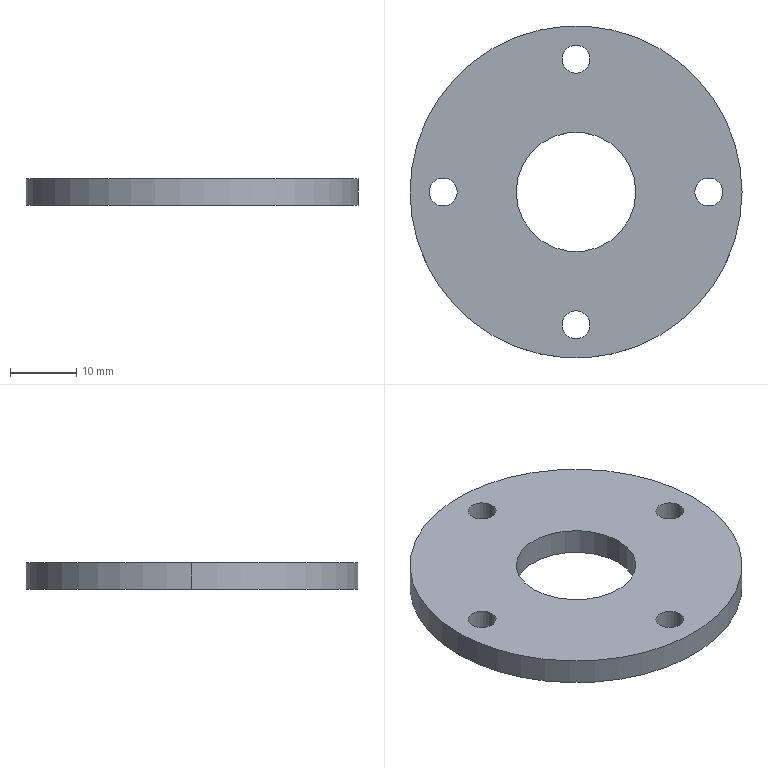Part | SolidWorks | features Extrusion 1 | 1 solid | 14 faces | box 50 x 50 x 4 mm | volume 6614 mm3 | cylinder 12 | plane 2 | commonest cylinder face diameters 4.2 x8 18 x2 50 x2
STEP:
#1=CARTESIAN_POINT('',(-2.1,-20.,4.));
#2=VERTEX_POINT('',#1);
#3=CARTESIAN_POINT('',(2.1,-20.,4.));
#4=VERTEX_POINT('',#3);
#5=CARTESIAN_POINT('',(0.,-20.,4.));
#6=DIRECTION('',(0.,0.,1.));
#7=DIRECTION('',(1.,0.,0.));
#8=AXIS2_PLACEMENT_3D('',#5,#6,#7);
#9=CIRCLE('',#8,2.1);
#10=EDGE_CURVE('',#2,#4,#9,.T.);
#11=ORIENTED_EDGE('',*,*,#10,.T.);
#12=CARTESIAN_POINT('',(2.1,-20.,0.));
#13=VERTEX_POINT('',#12);
#14=CARTESIAN_POINT('',(2.1,-20.,4.));
#15=DIRECTION('',(0.,0.,-1.));
#16=VECTOR('',#15,1000.);
#17=LINE('',#14,#16);
#18=EDGE_CURVE('',#4,#13,#17,.T.);
#19=ORIENTED_EDGE('',*,*,#18,.T.);
#20=CARTESIAN_POINT('',(-2.1,-20.,0.));
#21=VERTEX_POINT('',#20);
#22=CARTESIAN_POINT('',(0.,-20.,0.));
#23=DIRECTION('',(0.,0.,1.));
#24=DIRECTION('',(1.,0.,0.));
#25=AXIS2_PLACEMENT_3D('',#22,#23,#24);
#26=CIRCLE('',#25,2.1);
#27=EDGE_CURVE('',#21,#13,#26,.T.);
#28=ORIENTED_EDGE('',*,*,#27,.F.);
#29=CARTESIAN_POINT('',(-2.1,-20.,4.));
#30=DIRECTION('',(0.,0.,-1.));
#31=VECTOR('',#30,1000.);
#32=LINE('',#29,#31);
#33=EDGE_CURVE('',#2,#21,#32,.T.);
#34=ORIENTED_EDGE('',*,*,#33,.F.);
#35=EDGE_LOOP('',(#11,#19,#28,#34));
#36=FACE_OUTER_BOUND('',#35,.T.);
#37=CARTESIAN_POINT('',(0.,-20.,4.));
#38=DIRECTION('',(0.,0.,-1.));
#39=DIRECTION('',(-1.,0.,0.));
#40=AXIS2_PLACEMENT_3D('',#37,#38,#39);
#41=CYLINDRICAL_SURFACE('',#40,2.1);
#42=ADVANCED_FACE('',(#36),#41,.F.);
#43=CARTESIAN_POINT('',(17.9,0.,4.));
#44=VERTEX_POINT('',#43);
#45=CARTESIAN_POINT('',(22.1,0.,4.));
#46=VERTEX_POINT('',#45);
#47=CARTESIAN_POINT('',(20.,0.,4.));
#48=DIRECTION('',(0.,0.,1.));
#49=DIRECTION('',(1.,0.,0.));
#50=AXIS2_PLACEMENT_3D('',#47,#48,#49);
#51=CIRCLE('',#50,2.1);
#52=EDGE_CURVE('',#44,#46,#51,.T.);
#53=ORIENTED_EDGE('',*,*,#52,.T.);
#54=CARTESIAN_POINT('',(22.1,0.,0.));
#55=VERTEX_POINT('',#54);
#56=CARTESIAN_POINT('',(22.1,0.,4.));
#57=DIRECTION('',(0.,0.,-1.));
#58=VECTOR('',#57,1000.);
#59=LINE('',#56,#58);
#60=EDGE_CURVE('',#46,#55,#59,.T.);
#61=ORIENTED_EDGE('',*,*,#60,.T.);
#62=CARTESIAN_POINT('',(17.9,0.,0.));
#63=VERTEX_POINT('',#62);
#64=CARTESIAN_POINT('',(20.,0.,0.));
#65=DIRECTION('',(0.,0.,1.));
#66=DIRECTION('',(1.,0.,0.));
#67=AXIS2_PLACEMENT_3D('',#64,#65,#66);
#68=CIRCLE('',#67,2.1);
#69=EDGE_CURVE('',#63,#55,#68,.T.);
#70=ORIENTED_EDGE('',*,*,#69,.F.);
#71=CARTESIAN_POINT('',(17.9,0.,4.));
#72=DIRECTION('',(0.,0.,-1.));
#73=VECTOR('',#72,1000.);
#74=LINE('',#71,#73);
#75=EDGE_CURVE('',#44,#63,#74,.T.);
#76=ORIENTED_EDGE('',*,*,#75,.F.);
#77=EDGE_LOOP('',(#53,#61,#70,#76));
#78=FACE_OUTER_BOUND('',#77,.T.);
#79=CARTESIAN_POINT('',(20.,0.,4.));
#80=DIRECTION('',(0.,0.,-1.));
#81=DIRECTION('',(-1.,0.,0.));
#82=AXIS2_PLACEMENT_3D('',#79,#80,#81);
#83=CYLINDRICAL_SURFACE('',#82,2.1);
#84=ADVANCED_FACE('',(#78),#83,.F.);
#85=CARTESIAN_POINT('',(-22.1,0.,4.));
#86=VERTEX_POINT('',#85);
#87=CARTESIAN_POINT('',(-17.9,0.,4.));
#88=VERTEX_POINT('',#87);
#89=CARTESIAN_POINT('',(-20.,0.,4.));
#90=DIRECTION('',(0.,0.,1.));
#91=DIRECTION('',(1.,0.,0.));
#92=AXIS2_PLACEMENT_3D('',#89,#90,#91);
#93=CIRCLE('',#92,2.1);
#94=EDGE_CURVE('',#86,#88,#93,.T.);
#95=ORIENTED_EDGE('',*,*,#94,.T.);
#96=CARTESIAN_POINT('',(-17.9,0.,0.));
#97=VERTEX_POINT('',#96);
#98=CARTESIAN_POINT('',(-17.9,0.,4.));
#99=DIRECTION('',(0.,0.,-1.));
#100=VECTOR('',#99,1000.);
#101=LINE('',#98,#100);
#102=EDGE_CURVE('',#88,#97,#101,.T.);
#103=ORIENTED_EDGE('',*,*,#102,.T.);
#104=CARTESIAN_POINT('',(-22.1,0.,0.));
#105=VERTEX_POINT('',#104);
#106=CARTESIAN_POINT('',(-20.,0.,0.));
#107=DIRECTION('',(0.,0.,1.));
#108=DIRECTION('',(1.,0.,0.));
#109=AXIS2_PLACEMENT_3D('',#106,#107,#108);
#110=CIRCLE('',#109,2.1);
#111=EDGE_CURVE('',#105,#97,#110,.T.);
#112=ORIENTED_EDGE('',*,*,#111,.F.);
#113=CARTESIAN_POINT('',(-22.1,0.,4.));
#114=DIRECTION('',(0.,0.,-1.));
#115=VECTOR('',#114,1000.);
#116=LINE('',#113,#115);
#117=EDGE_CURVE('',#86,#105,#116,.T.);
#118=ORIENTED_EDGE('',*,*,#117,.F.);
#119=EDGE_LOOP('',(#95,#103,#112,#118));
#120=FACE_OUTER_BOUND('',#119,.T.);
#121=CARTESIAN_POINT('',(-20.,0.,4.));
#122=DIRECTION('',(0.,0.,-1.));
#123=DIRECTION('',(-1.,0.,0.));
#124=AXIS2_PLACEMENT_3D('',#121,#122,#123);
#125=CYLINDRICAL_SURFACE('',#124,2.1);
#126=ADVANCED_FACE('',(#120),#125,.F.);
#127=CARTESIAN_POINT('',(-2.1,20.,4.));
#128=VERTEX_POINT('',#127);
#129=CARTESIAN_POINT('',(2.1,20.,4.));
#130=VERTEX_POINT('',#129);
#131=CARTESIAN_POINT('',(0.,20.,4.));
#132=DIRECTION('',(0.,0.,1.));
#133=DIRECTION('',(1.,0.,0.));
#134=AXIS2_PLACEMENT_3D('',#131,#132,#133);
#135=CIRCLE('',#134,2.1);
#136=EDGE_CURVE('',#128,#130,#135,.T.);
#137=ORIENTED_EDGE('',*,*,#136,.T.);
#138=CARTESIAN_POINT('',(2.1,20.,0.));
#139=VERTEX_POINT('',#138);
#140=CARTESIAN_POINT('',(2.1,20.,4.));
#141=DIRECTION('',(0.,0.,-1.));
#142=VECTOR('',#141,1000.);
#143=LINE('',#140,#142);
#144=EDGE_CURVE('',#130,#139,#143,.T.);
#145=ORIENTED_EDGE('',*,*,#144,.T.);
#146=CARTESIAN_POINT('',(-2.1,20.,0.));
#147=VERTEX_POINT('',#146);
#148=CARTESIAN_POINT('',(0.,20.,0.));
#149=DIRECTION('',(0.,0.,1.));
#150=DIRECTION('',(1.,0.,0.));
#151=AXIS2_PLACEMENT_3D('',#148,#149,#150);
#152=CIRCLE('',#151,2.1);
#153=EDGE_CURVE('',#147,#139,#152,.T.);
#154=ORIENTED_EDGE('',*,*,#153,.F.);
#155=CARTESIAN_POINT('',(-2.1,20.,4.));
#156=DIRECTION('',(0.,0.,-1.));
#157=VECTOR('',#156,1000.);
#158=LINE('',#155,#157);
#159=EDGE_CURVE('',#128,#147,#158,.T.);
#160=ORIENTED_EDGE('',*,*,#159,.F.);
#161=EDGE_LOOP('',(#137,#145,#154,#160));
#162=FACE_OUTER_BOUND('',#161,.T.);
#163=CARTESIAN_POINT('',(0.,20.,4.));
#164=DIRECTION('',(0.,0.,-1.));
#165=DIRECTION('',(-1.,0.,0.));
#166=AXIS2_PLACEMENT_3D('',#163,#164,#165);
#167=CYLINDRICAL_SURFACE('',#166,2.1);
#168=ADVANCED_FACE('',(#162),#167,.F.);
#169=CARTESIAN_POINT('',(-9.,0.,4.));
#170=VERTEX_POINT('',#169);
#171=CARTESIAN_POINT('',(9.,0.,4.));
#172=VERTEX_POINT('',#171);
#173=CARTESIAN_POINT('',(0.,0.,4.));
#174=DIRECTION('',(0.,0.,1.));
#175=DIRECTION('',(1.,0.,0.));
#176=AXIS2_PLACEMENT_3D('',#173,#174,#175);
#177=CIRCLE('',#176,9.);
#178=EDGE_CURVE('',#170,#172,#177,.T.);
#179=ORIENTED_EDGE('',*,*,#178,.T.);
#180=CARTESIAN_POINT('',(9.,0.,0.));
#181=VERTEX_POINT('',#180);
#182=CARTESIAN_POINT('',(9.,0.,4.));
#183=DIRECTION('',(0.,0.,-1.));
#184=VECTOR('',#183,1000.);
#185=LINE('',#182,#184);
#186=EDGE_CURVE('',#172,#181,#185,.T.);
#187=ORIENTED_EDGE('',*,*,#186,.T.);
#188=CARTESIAN_POINT('',(-9.,0.,0.));
#189=VERTEX_POINT('',#188);
#190=CARTESIAN_POINT('',(0.,0.,0.));
#191=DIRECTION('',(0.,0.,1.));
#192=DIRECTION('',(1.,0.,0.));
#193=AXIS2_PLACEMENT_3D('',#190,#191,#192);
#194=CIRCLE('',#193,9.);
#195=EDGE_CURVE('',#189,#181,#194,.T.);
#196=ORIENTED_EDGE('',*,*,#195,.F.);
#197=CARTESIAN_POINT('',(-9.,0.,4.));
#198=DIRECTION('',(0.,0.,-1.));
#199=VECTOR('',#198,1000.);
#200=LINE('',#197,#199);
#201=EDGE_CURVE('',#170,#189,#200,.T.);
#202=ORIENTED_EDGE('',*,*,#201,.F.);
#203=EDGE_LOOP('',(#179,#187,#196,#202));
#204=FACE_OUTER_BOUND('',#203,.T.);
#205=CARTESIAN_POINT('',(0.,0.,4.));
#206=DIRECTION('',(0.,0.,-1.));
#207=DIRECTION('',(-1.,0.,0.));
#208=AXIS2_PLACEMENT_3D('',#205,#206,#207);
#209=CYLINDRICAL_SURFACE('',#208,9.);
#210=ADVANCED_FACE('',(#204),#209,.F.);
#211=CARTESIAN_POINT('',(25.,0.,4.));
#212=VERTEX_POINT('',#211);
#213=CARTESIAN_POINT('',(-25.,0.,4.));
#214=VERTEX_POINT('',#213);
#215=CARTESIAN_POINT('',(0.,0.,4.));
#216=DIRECTION('',(0.,0.,1.));
#217=DIRECTION('',(1.,0.,0.));
#218=AXIS2_PLACEMENT_3D('',#215,#216,#217);
#219=CIRCLE('',#218,25.);
#220=EDGE_CURVE('',#212,#214,#219,.T.);
#221=ORIENTED_EDGE('',*,*,#220,.F.);
#222=CARTESIAN_POINT('',(25.,0.,0.));
#223=VERTEX_POINT('',#222);
#224=CARTESIAN_POINT('',(25.,0.,4.));
#225=DIRECTION('',(0.,0.,-1.));
#226=VECTOR('',#225,1000.);
#227=LINE('',#224,#226);
#228=EDGE_CURVE('',#212,#223,#227,.T.);
#229=ORIENTED_EDGE('',*,*,#228,.T.);
#230=CARTESIAN_POINT('',(-25.,0.,0.));
#231=VERTEX_POINT('',#230);
#232=CARTESIAN_POINT('',(0.,0.,0.));
#233=DIRECTION('',(0.,0.,1.));
#234=DIRECTION('',(1.,0.,0.));
#235=AXIS2_PLACEMENT_3D('',#232,#233,#234);
#236=CIRCLE('',#235,25.);
#237=EDGE_CURVE('',#223,#231,#236,.T.);
#238=ORIENTED_EDGE('',*,*,#237,.T.);
#239=CARTESIAN_POINT('',(-25.,0.,4.));
#240=DIRECTION('',(0.,0.,-1.));
#241=VECTOR('',#240,1000.);
#242=LINE('',#239,#241);
#243=EDGE_CURVE('',#214,#231,#242,.T.);
#244=ORIENTED_EDGE('',*,*,#243,.F.);
#245=EDGE_LOOP('',(#221,#229,#238,#244));
#246=FACE_OUTER_BOUND('',#245,.T.);
#247=CARTESIAN_POINT('',(0.,0.,4.));
#248=DIRECTION('',(0.,0.,-1.));
#249=DIRECTION('',(-1.,0.,0.));
#250=AXIS2_PLACEMENT_3D('',#247,#248,#249);
#251=CYLINDRICAL_SURFACE('',#250,25.);
#252=ADVANCED_FACE('',(#246),#251,.T.);
#253=ORIENTED_EDGE('',*,*,#52,.F.);
#254=CARTESIAN_POINT('',(20.,0.,4.));
#255=DIRECTION('',(0.,0.,1.));
#256=DIRECTION('',(1.,0.,0.));
#257=AXIS2_PLACEMENT_3D('',#254,#255,#256);
#258=CIRCLE('',#257,2.1);
#259=EDGE_CURVE('',#46,#44,#258,.T.);
#260=ORIENTED_EDGE('',*,*,#259,.F.);
#261=EDGE_LOOP('',(#253,#260));
#262=FACE_BOUND('',#261,.T.);
#263=ORIENTED_EDGE('',*,*,#136,.F.);
#264=CARTESIAN_POINT('',(0.,20.,4.));
#265=DIRECTION('',(0.,0.,1.));
#266=DIRECTION('',(1.,0.,0.));
#267=AXIS2_PLACEMENT_3D('',#264,#265,#266);
#268=CIRCLE('',#267,2.1);
#269=EDGE_CURVE('',#130,#128,#268,.T.);
#270=ORIENTED_EDGE('',*,*,#269,.F.);
#271=EDGE_LOOP('',(#263,#270));
#272=FACE_BOUND('',#271,.T.);
#273=CARTESIAN_POINT('',(0.,0.,4.));
#274=DIRECTION('',(0.,0.,1.));
#275=DIRECTION('',(1.,0.,0.));
#276=AXIS2_PLACEMENT_3D('',#273,#274,#275);
#277=CIRCLE('',#276,25.);
#278=EDGE_CURVE('',#214,#212,#277,.T.);
#279=ORIENTED_EDGE('',*,*,#278,.T.);
#280=ORIENTED_EDGE('',*,*,#220,.T.);
#281=EDGE_LOOP('',(#279,#280));
#282=FACE_OUTER_BOUND('',#281,.T.);
#283=ORIENTED_EDGE('',*,*,#178,.F.);
#284=CARTESIAN_POINT('',(0.,0.,4.));
#285=DIRECTION('',(0.,0.,1.));
#286=DIRECTION('',(1.,0.,0.));
#287=AXIS2_PLACEMENT_3D('',#284,#285,#286);
#288=CIRCLE('',#287,9.);
#289=EDGE_CURVE('',#172,#170,#288,.T.);
#290=ORIENTED_EDGE('',*,*,#289,.F.);
#291=EDGE_LOOP('',(#283,#290));
#292=FACE_BOUND('',#291,.T.);
#293=ORIENTED_EDGE('',*,*,#94,.F.);
#294=CARTESIAN_POINT('',(-20.,0.,4.));
#295=DIRECTION('',(0.,0.,1.));
#296=DIRECTION('',(1.,0.,0.));
#297=AXIS2_PLACEMENT_3D('',#294,#295,#296);
#298=CIRCLE('',#297,2.1);
#299=EDGE_CURVE('',#88,#86,#298,.T.);
#300=ORIENTED_EDGE('',*,*,#299,.F.);
#301=EDGE_LOOP('',(#293,#300));
#302=FACE_BOUND('',#301,.T.);
#303=ORIENTED_EDGE('',*,*,#10,.F.);
#304=CARTESIAN_POINT('',(0.,-20.,4.));
#305=DIRECTION('',(0.,0.,1.));
#306=DIRECTION('',(1.,0.,0.));
#307=AXIS2_PLACEMENT_3D('',#304,#305,#306);
#308=CIRCLE('',#307,2.1);
#309=EDGE_CURVE('',#4,#2,#308,.T.);
#310=ORIENTED_EDGE('',*,*,#309,.F.);
#311=EDGE_LOOP('',(#303,#310));
#312=FACE_BOUND('',#311,.T.);
#313=CARTESIAN_POINT('',(0.,0.,4.));
#314=DIRECTION('',(0.,0.,1.));
#315=DIRECTION('',(1.,0.,0.));
#316=AXIS2_PLACEMENT_3D('',#313,#314,#315);
#317=PLANE('',#316);
#318=ADVANCED_FACE('',(#262,#272,#282,#292,#302,#312),#317,.T.);
#319=CARTESIAN_POINT('',(0.,0.,0.));
#320=DIRECTION('',(0.,0.,1.));
#321=DIRECTION('',(1.,0.,0.));
#322=AXIS2_PLACEMENT_3D('',#319,#320,#321);
#323=CIRCLE('',#322,25.);
#324=EDGE_CURVE('',#231,#223,#323,.T.);
#325=ORIENTED_EDGE('',*,*,#324,.F.);
#326=ORIENTED_EDGE('',*,*,#237,.F.);
#327=EDGE_LOOP('',(#325,#326));
#328=FACE_OUTER_BOUND('',#327,.T.);
#329=ORIENTED_EDGE('',*,*,#195,.T.);
#330=CARTESIAN_POINT('',(0.,0.,0.));
#331=DIRECTION('',(0.,0.,1.));
#332=DIRECTION('',(1.,0.,0.));
#333=AXIS2_PLACEMENT_3D('',#330,#331,#332);
#334=CIRCLE('',#333,9.);
#335=EDGE_CURVE('',#181,#189,#334,.T.);
#336=ORIENTED_EDGE('',*,*,#335,.T.);
#337=EDGE_LOOP('',(#329,#336));
#338=FACE_BOUND('',#337,.T.);
#339=ORIENTED_EDGE('',*,*,#153,.T.);
#340=CARTESIAN_POINT('',(0.,20.,0.));
#341=DIRECTION('',(0.,0.,1.));
#342=DIRECTION('',(1.,0.,0.));
#343=AXIS2_PLACEMENT_3D('',#340,#341,#342);
#344=CIRCLE('',#343,2.1);
#345=EDGE_CURVE('',#139,#147,#344,.T.);
#346=ORIENTED_EDGE('',*,*,#345,.T.);
#347=EDGE_LOOP('',(#339,#346));
#348=FACE_BOUND('',#347,.T.);
#349=ORIENTED_EDGE('',*,*,#111,.T.);
#350=CARTESIAN_POINT('',(-20.,0.,0.));
#351=DIRECTION('',(0.,0.,1.));
#352=DIRECTION('',(1.,0.,0.));
#353=AXIS2_PLACEMENT_3D('',#350,#351,#352);
#354=CIRCLE('',#353,2.1);
#355=EDGE_CURVE('',#97,#105,#354,.T.);
#356=ORIENTED_EDGE('',*,*,#355,.T.);
#357=EDGE_LOOP('',(#349,#356));
#358=FACE_BOUND('',#357,.T.);
#359=ORIENTED_EDGE('',*,*,#69,.T.);
#360=CARTESIAN_POINT('',(20.,0.,0.));
#361=DIRECTION('',(0.,0.,1.));
#362=DIRECTION('',(1.,0.,0.));
#363=AXIS2_PLACEMENT_3D('',#360,#361,#362);
#364=CIRCLE('',#363,2.1);
#365=EDGE_CURVE('',#55,#63,#364,.T.);
#366=ORIENTED_EDGE('',*,*,#365,.T.);
#367=EDGE_LOOP('',(#359,#366));
#368=FACE_BOUND('',#367,.T.);
#369=ORIENTED_EDGE('',*,*,#27,.T.);
#370=CARTESIAN_POINT('',(0.,-20.,0.));
#371=DIRECTION('',(0.,0.,1.));
#372=DIRECTION('',(1.,0.,0.));
#373=AXIS2_PLACEMENT_3D('',#370,#371,#372);
#374=CIRCLE('',#373,2.1);
#375=EDGE_CURVE('',#13,#21,#374,.T.);
#376=ORIENTED_EDGE('',*,*,#375,.T.);
#377=EDGE_LOOP('',(#369,#376));
#378=FACE_BOUND('',#377,.T.);
#379=CARTESIAN_POINT('',(0.,0.,0.));
#380=DIRECTION('',(0.,0.,1.));
#381=DIRECTION('',(1.,0.,0.));
#382=AXIS2_PLACEMENT_3D('',#379,#380,#381);
#383=PLANE('',#382);
#384=ADVANCED_FACE('',(#328,#338,#348,#358,#368,#378),#383,.F.);
#385=ORIENTED_EDGE('',*,*,#228,.F.);
#386=ORIENTED_EDGE('',*,*,#278,.F.);
#387=ORIENTED_EDGE('',*,*,#243,.T.);
#388=ORIENTED_EDGE('',*,*,#324,.T.);
#389=EDGE_LOOP('',(#385,#386,#387,#388));
#390=FACE_OUTER_BOUND('',#389,.T.);
#391=CARTESIAN_POINT('',(0.,0.,4.));
#392=DIRECTION('',(0.,0.,-1.));
#393=DIRECTION('',(-1.,0.,0.));
#394=AXIS2_PLACEMENT_3D('',#391,#392,#393);
#395=CYLINDRICAL_SURFACE('',#394,25.);
#396=ADVANCED_FACE('',(#390),#395,.T.);
#397=ORIENTED_EDGE('',*,*,#186,.F.);
#398=ORIENTED_EDGE('',*,*,#289,.T.);
#399=ORIENTED_EDGE('',*,*,#201,.T.);
#400=ORIENTED_EDGE('',*,*,#335,.F.);
#401=EDGE_LOOP('',(#397,#398,#399,#400));
#402=FACE_OUTER_BOUND('',#401,.T.);
#403=CARTESIAN_POINT('',(0.,0.,4.));
#404=DIRECTION('',(0.,0.,-1.));
#405=DIRECTION('',(-1.,0.,0.));
#406=AXIS2_PLACEMENT_3D('',#403,#404,#405);
#407=CYLINDRICAL_SURFACE('',#406,9.);
#408=ADVANCED_FACE('',(#402),#407,.F.);
#409=ORIENTED_EDGE('',*,*,#144,.F.);
#410=ORIENTED_EDGE('',*,*,#269,.T.);
#411=ORIENTED_EDGE('',*,*,#159,.T.);
#412=ORIENTED_EDGE('',*,*,#345,.F.);
#413=EDGE_LOOP('',(#409,#410,#411,#412));
#414=FACE_OUTER_BOUND('',#413,.T.);
#415=CARTESIAN_POINT('',(0.,20.,4.));
#416=DIRECTION('',(0.,0.,-1.));
#417=DIRECTION('',(-1.,0.,0.));
#418=AXIS2_PLACEMENT_3D('',#415,#416,#417);
#419=CYLINDRICAL_SURFACE('',#418,2.1);
#420=ADVANCED_FACE('',(#414),#419,.F.);
#421=ORIENTED_EDGE('',*,*,#102,.F.);
#422=ORIENTED_EDGE('',*,*,#299,.T.);
#423=ORIENTED_EDGE('',*,*,#117,.T.);
#424=ORIENTED_EDGE('',*,*,#355,.F.);
#425=EDGE_LOOP('',(#421,#422,#423,#424));
#426=FACE_OUTER_BOUND('',#425,.T.);
#427=CARTESIAN_POINT('',(-20.,0.,4.));
#428=DIRECTION('',(0.,0.,-1.));
#429=DIRECTION('',(-1.,0.,0.));
#430=AXIS2_PLACEMENT_3D('',#427,#428,#429);
#431=CYLINDRICAL_SURFACE('',#430,2.1);
#432=ADVANCED_FACE('',(#426),#431,.F.);
#433=ORIENTED_EDGE('',*,*,#60,.F.);
#434=ORIENTED_EDGE('',*,*,#259,.T.);
#435=ORIENTED_EDGE('',*,*,#75,.T.);
#436=ORIENTED_EDGE('',*,*,#365,.F.);
#437=EDGE_LOOP('',(#433,#434,#435,#436));
#438=FACE_OUTER_BOUND('',#437,.T.);
#439=CARTESIAN_POINT('',(20.,0.,4.));
#440=DIRECTION('',(0.,0.,-1.));
#441=DIRECTION('',(-1.,0.,0.));
#442=AXIS2_PLACEMENT_3D('',#439,#440,#441);
#443=CYLINDRICAL_SURFACE('',#442,2.1);
#444=ADVANCED_FACE('',(#438),#443,.F.);
#445=ORIENTED_EDGE('',*,*,#18,.F.);
#446=ORIENTED_EDGE('',*,*,#309,.T.);
#447=ORIENTED_EDGE('',*,*,#33,.T.);
#448=ORIENTED_EDGE('',*,*,#375,.F.);
#449=EDGE_LOOP('',(#445,#446,#447,#448));
#450=FACE_OUTER_BOUND('',#449,.T.);
#451=CARTESIAN_POINT('',(0.,-20.,4.));
#452=DIRECTION('',(0.,0.,-1.));
#453=DIRECTION('',(-1.,0.,0.));
#454=AXIS2_PLACEMENT_3D('',#451,#452,#453);
#455=CYLINDRICAL_SURFACE('',#454,2.1);
#456=ADVANCED_FACE('',(#450),#455,.F.);
#457=CLOSED_SHELL('',(#42,#84,#126,#168,#210,#252,#318,#384,#396,#408,#420,#432,#444,#456));
#458=MANIFOLD_SOLID_BREP('',#457);
#459=CARTESIAN_POINT('',(0.,0.,0.));
#460=DIRECTION('',(0.,0.,1.));
#461=DIRECTION('',(1.,0.,0.));
#462=AXIS2_PLACEMENT_3D('',#459,#460,#461);
#463=(LENGTH_UNIT()NAMED_UNIT(*)SI_UNIT(.MILLI.,.METRE.));
#464=UNCERTAINTY_MEASURE_WITH_UNIT(LENGTH_MEASURE(0.00001),#463,'','');
#465=(NAMED_UNIT(*)PLANE_ANGLE_UNIT()SI_UNIT($,.RADIAN.));
#466=(NAMED_UNIT(*)SI_UNIT($,.STERADIAN.)SOLID_ANGLE_UNIT());
#467=(GEOMETRIC_REPRESENTATION_CONTEXT(3)GLOBAL_UNCERTAINTY_ASSIGNED_CONTEXT((#464))GLOBAL_UNIT_ASSIGNED_CONTEXT((#463,#465,#466))REPRESENTATION_CONTEXT('',''));
#468=ADVANCED_BREP_SHAPE_REPRESENTATION('',(#458,#462),#467);